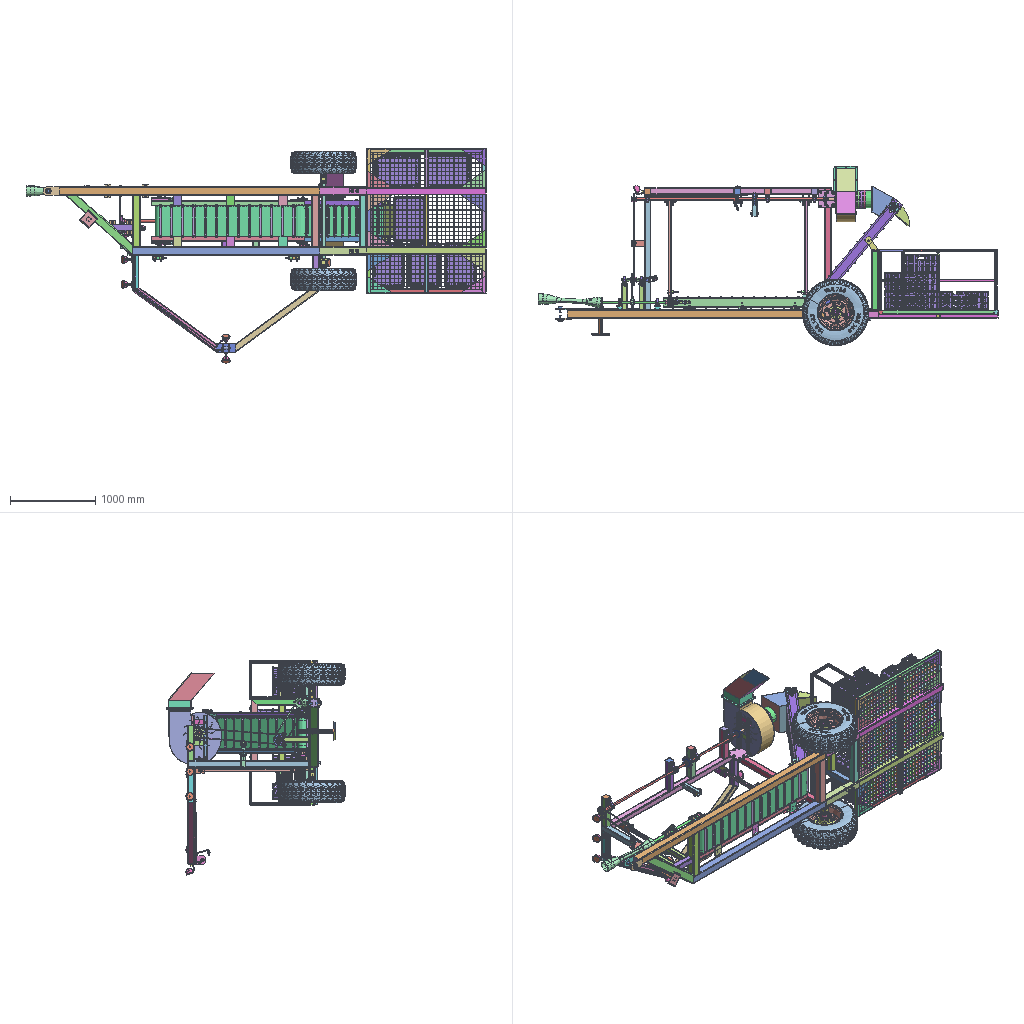Assembly | STEP file | 149 different items | 1323 placed | box 5395 x 2101 x 2512 mm
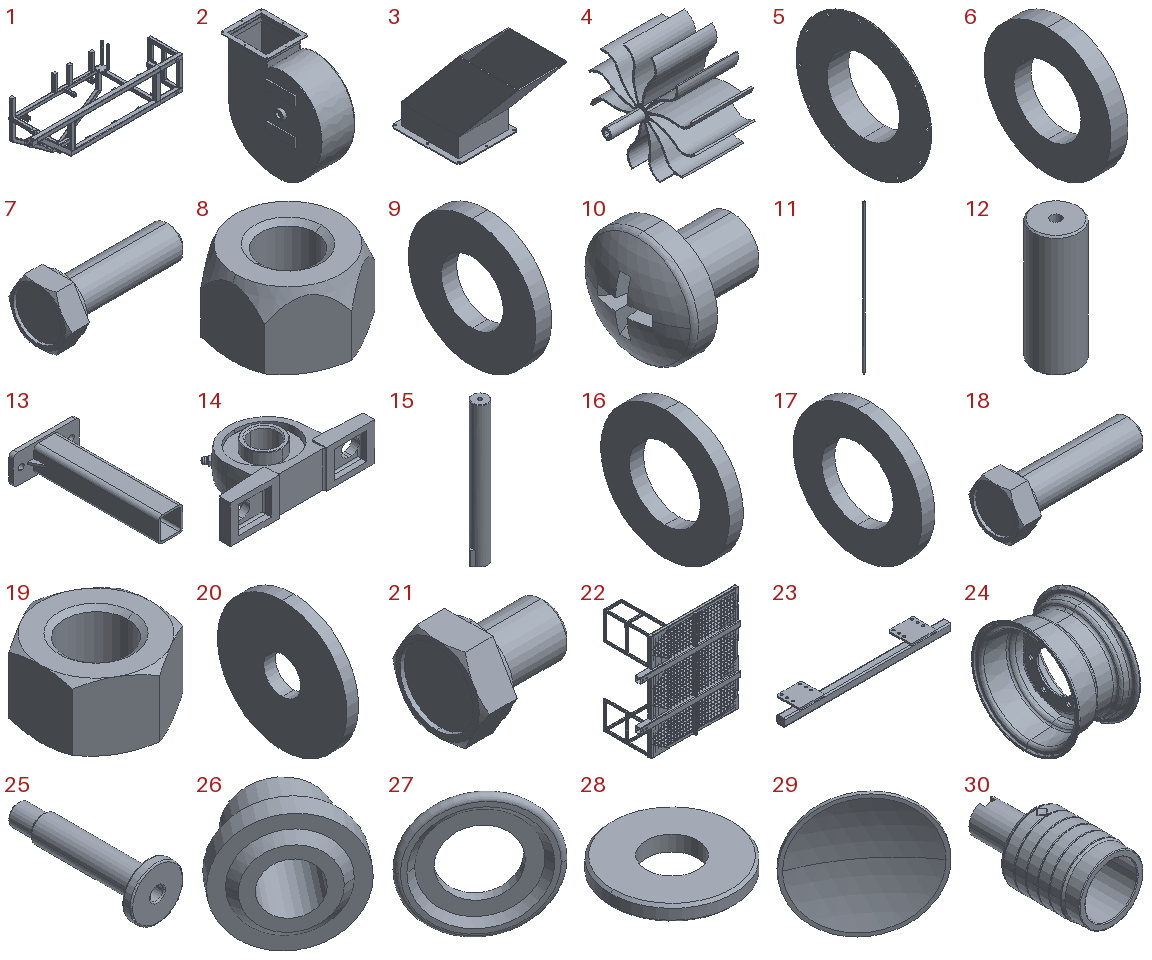Parts list (item | name | quantity | parent item | size | volume):
1 | 01_GLOWNA_RAMAV11_Default<Obrobiona> | x1 | in MAIN_FRAME_ASSEMBLY1V11 | 3794 x 1545 x 1980 mm | 40557701 mm3
2 | wentylator 1V11 | x1 | in ASSEMBLY_WENTYLATOR1V11 | 280 x 648.901 x 670.864 mm | 4184150 mm3
3 | odciag11V11 | x1 | in ASSEMBLY_WENTYLATOR1V11 | 280 x 560.788 x 414.862 mm | 1890664 mm3
4 | lopatki1V11 | x1 | in ASSEMBLY_WENTYLATOR1V11 | 347 x 377.952 x 377.952 mm | 3263464 mm3
5 | wentylator blacha dodatkowaV11 | x1 | in ASSEMBLY_WENTYLATOR1V11 | 60 x 370 x 370 mm | 388519 mm3
6 | flat washer narrow_am_B18.22M - Plain washer, 6 mm, narrow | x16 | in ASSEMBLY_WENTYLATOR1V11 | 1.75 x 13 x 13 mm | 167.412 mm3
7 | formed hex screw_am_B18.2.3.2M - Formed hex screw, M6 x 1.0 x 20 --20WN | x8 | in ASSEMBLY_WENTYLATOR1V11 | 24.15 x 11.547 x 10 mm | 885.854 mm3
8 | prevailing torque hex nut_am_AM-M6-N | x10 | in ASSEMBLY_WENTYLATOR1V11, P01_ASSEMBLY_FRUIT_HARVESTER1 | 10 x 11.547 x 6.7 mm | 433.135 mm3
9 | flat washer narrow_am_B18.22M - Plain washer, 8 mm, narrow | x12 | in ASSEMBLY_WENTYLATOR1V11 | 2.3 x 18.8 x 18.8 mm | 488.212 mm3
10 | pan cross head_am_B18.6.7M - M8 x 1.25 x 10 Type I Cross Recessed PHMS --10N | x12 | in ASSEMBLY_WENTYLATOR1V11 | 15.946 x 16 x 16 mm | 1390 mm3
11 | Shaft dia30 2280V11 | x1 | in MAIN_FRAME_ASSEMBLY1V11 | 30 x 30 x 2310 mm | 1619744 mm3
12 | SHAFT_DIA30_80V11 | x1 | in MAIN_FRAME_ASSEMBLY1V11 | 30 x 30 x 80 mm | 54791 mm3
13 | MOUNTING_BOTTOM_PROFILEV11_Default<Machined> | x2 | in ASSEMBLY_MOCOWANIE1V11 | 160 x 310 x 70 mm | 420999 mm3
14 | ucp206_01V11 | x4 | in ASSEMBLY_MOCOWANIE1V11, ASSEMBLY_MOCOWANIE2V11 | 160 x 84 x 43.2 mm | 181107 mm3
15 | SHAFT_DIA30_BOTTOM_MOUNTINGV11 | x1 | in ASSEMBLY_MOCOWANIE1V11 | 39 x 30 x 270 mm | 190340 mm3
16 | flat washer narrow_am_B18.22M - Plain washer, 16 mm, narrow | x5 | in ASSEMBLY_MOCOWANIE1V11, zlozenie mniejszego podajnika1V11 | 3.5 x 32 x 32 mm | 1956 mm3
17 | flat washer narrow_am_B18.22M - Plain washer, 14 mm, narrow | x56 | in ASSEMBLY_MOCOWANIE1V11, Assembly Ucp206V11, MAIN_FRAME_ASSEMBLY1V11, ASSEMBLY_MOCOWANIE2V11 | 2.8 x 28 x 28 mm | 1194 mm3
18 | formed hex screw_am_B18.2.3.2M - Formed hex screw, M14 x 2.0 x 50 --34WN | x4 | in ASSEMBLY_MOCOWANIE1V11 | 59.09 x 24.249 x 21 mm | 10811 mm3
19 | hex nut style 1_am_B18.2.4.1M - Hex nut, Style 1,  M14 x 2 --D-N | x16 | in ASSEMBLY_MOCOWANIE1V11, MAIN_FRAME_ASSEMBLY1V11 | 21 x 24.249 x 12.8 mm | 3392 mm3
20 | flat washer wide_am_B18.22M - Plain washer, 10 mm, wide | x1 | in ASSEMBLY_MOCOWANIE1V11 | 3.5 x 39 x 39 mm | 3841 mm3
21 | formed hex screw_am_B18.2.3.2M - Formed hex screw, M10 x 1.5 x 14 --14WN | x11 | in ASSEMBLY_MOCOWANIE1V11, zlozenie mniejszego podajnika1V11, P01_ASSEMBLY_FRUIT_HARVESTER1 | 20.63 x 18.475 x 16 mm | 2415 mm3
22 | REAR_RECEIVING_PLATFORMV11_Default<Machined> | x1 | in MAIN_FRAME_ASSEMBLY1V11 | 1600 x 805 x 1690 mm | 26046895 mm3
23 | REAR_AXIS_PROFILEV11_Default<Machined> | x1 | in REAR_AXIS_ASSEMBLY1V11 | 1070 x 150 x 60 mm | 1274604 mm3
24 | FELGA_9.00x15.3V11 | x2 | in GEAR_ASSEMBLYV11 | 254.399 x 439.355 x 439.355 mm | 2312376 mm3
25 | VALVE_1PARTV11 | x2 | in GEAR_ASSEMBLYV11 | 20 x 53 x 20 mm | 3450 mm3
26 | VALVE_2PARTV11 | x2 | in GEAR_ASSEMBLYV11 | 22.76 x 21.764 x 22 mm | 2471 mm3
27 | VALVE_3PARTV11 | x2 | in GEAR_ASSEMBLYV11 | 16.078 x 12.89 x 20 mm | 326.438 mm3
28 | VALVE_4PARTV11 | x2 | in GEAR_ASSEMBLYV11 | 24 x 24 x 3 mm | 1103 mm3
29 | VALVE_5PARTV11 | x2 | in GEAR_ASSEMBLYV11 | 5.639 x 4.467 x 7 mm | 24.483 mm3
30 | VALVE_6PARTV11 | x2 | in GEAR_ASSEMBLYV11 | 9 x 17 x 9 mm | 343.749 mm3
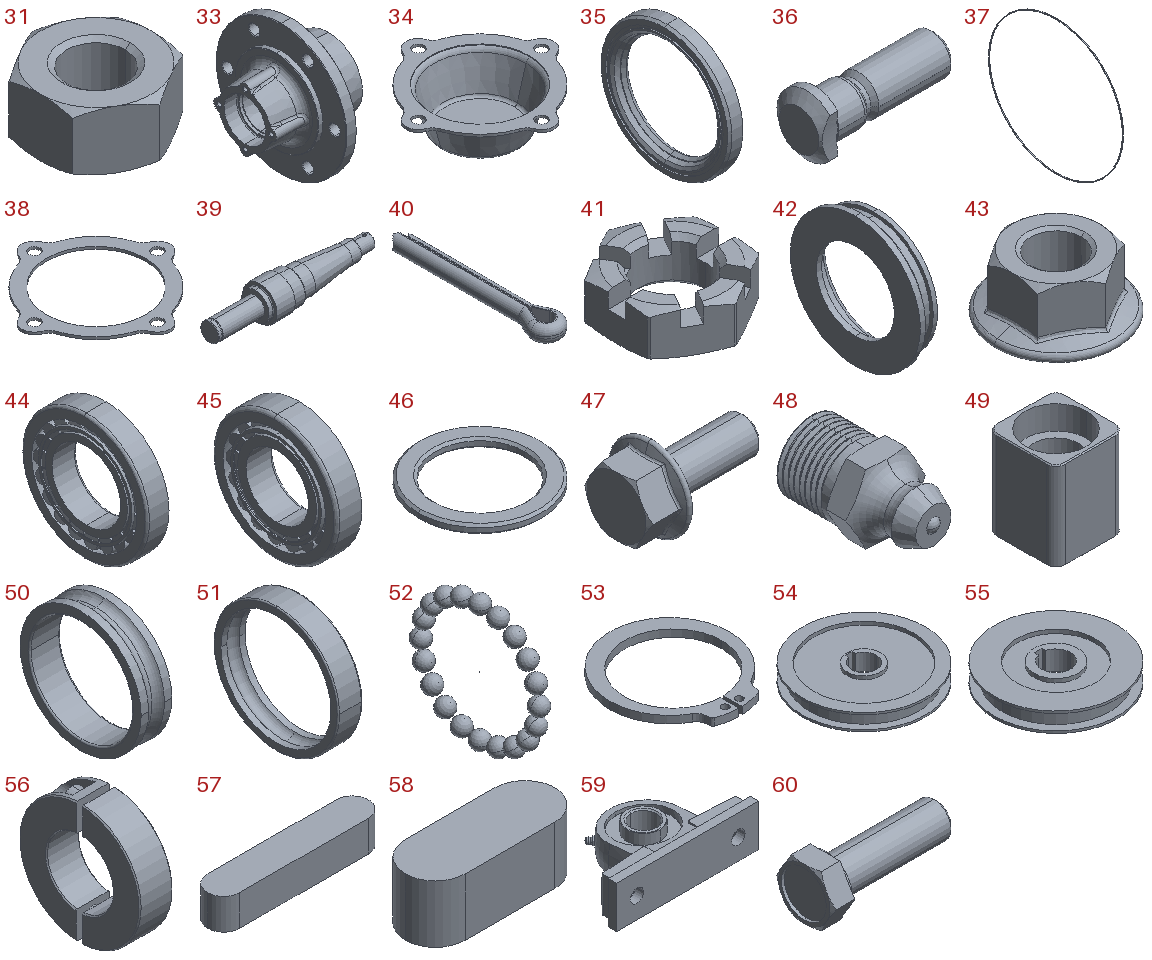31 | hex nut style 1_am_B18.2.4.1M - Hex nut, Style 1,  M10 x 1.5, with 16mm WAF --D-N | x2 | in GEAR_ASSEMBLYV11 | 16 x 18.475 x 8.4 mm | 1365 mm3
32 | OPONA_10.0-75_15.3V11 | x2 | in GEAR_ASSEMBLYV11 | - | -
33 | AXIS_HOUSING1V11 | x2 | in GEAR_ASSEMBLYV11 | 160 x 250 x 250 mm | 1786863 mm3
34 | AXIS_COVER1V11 | x2 | in GEAR_ASSEMBLYV11 | 120 x 120 x 31.5 mm | 20879 mm3
35 | SIMMERING_KORPUS1V11 | x2 | in GEAR_ASSEMBLYV11 | 10 x 95 x 95 mm | 14984 mm3
36 | SCREW_1SHAFTV11 | x12 | in GEAR_ASSEMBLYV11 | 68 x 26.359 x 30 mm | 23158 mm3
37 | USZCZELKA_SIMMERING1V11 | x2 | in GEAR_ASSEMBLYV11 | 0.5 x 78.541 x 78.541 mm | 35.939 mm3
38 | USZCZELKA1V11 | x2 | in GEAR_ASSEMBLYV11 | 120 x 120 x 2 mm | 6543 mm3
39 | SHAFT_AXIS_HOUSING1V11 | x2 | in GEAR_ASSEMBLYV11 | 349 x 75 x 75 mm | 734000 mm3
40 | SLIDER_SHAFT1V11 | x2 | in GEAR_ASSEMBLYV11 | 11.05 x 60.6 x 5.8 mm | 1645 mm3
41 | SHAFT_CAP1V11 | x2 | in GEAR_ASSEMBLYV11 | 46 x 52.616 x 18 mm | 18537 mm3
42 | AXIS_HOUSING_CLOSURE1V11 | x2 | in GEAR_ASSEMBLYV11 | 21 x 120 x 120 mm | 65717 mm3
43 | hex flange nut_am_B18.2.2.4M - Hex flange nut, M20 x 2.5 --N | x12 | in GEAR_ASSEMBLYV11 | 42.8 x 42.8 x 20 mm | 12973 mm3
44 | 30212V11 | x2 | in GEAR_ASSEMBLYV11 | 23.75 x 110 x 110 mm | 111845 mm3
45 | 30208V11 | x2 | in GEAR_ASSEMBLYV11 | 19.75 x 80 x 80 mm | 51729 mm3
46 | WASHER_DIA40_1V11 | x2 | in GEAR_ASSEMBLYV11 | 55 x 55 x 4 mm | 4178 mm3
47 | heavy hex flange screw_am_B18.2.3.9M - Heavy hex flange screw, M8 x 1.25 x 20 --20N | x8 | in GEAR_ASSEMBLYV11 | 28.1 x 18 x 18 mm | 2330 mm3
48 | KALAMITKA_1V11 | x2 | in GEAR_ASSEMBLYV11 | 11.547 x 18.49 x 10 mm | 633.492 mm3
49 | MILLED_BLOCK_FOR_AXISV11 | x2 | in REAR_AXIS_ASSEMBLY1V11 | 70 x 70 x 90 mm | 221300 mm3
50 | bearing_6908_01V11 | x8 | in bearing_6908V11 | 12 x 47.33 x 47.33 mm | 4895 mm3
51 | bearing_6908_02V11 | x8 | in bearing_6908V11 | 12 x 62 x 62 mm | 6668 mm3
52 | bearing_6908_03V11 | x8 | in bearing_6908V11 | 7.2 x 58.195 x 58.195 mm | 3909 mm3
53 | heavy duty external retaining ring_am_B27.8M - 3DM1-40 | x2 | in REAR_AXIS_ASSEMBLY1V11 | 46.312 x 50.391 x 2.8 mm | 1790 mm3
54 | Pulley 150 belt ha13v1V11 | x3 | in MAIN_FRAME_ASSEMBLY1V11 | 147 x 147 x 20 mm | 190388 mm3
55 | Pulley 150 belt ha13 v1V11 | x3 | in MAIN_FRAME_ASSEMBLY1V11, P01_ASSEMBLY_FRUIT_HARVESTER1 | 127 x 127 x 20 mm | 165003 mm3
56 | Split Shaft Collar_ Steel GN 707.2-55-B30-STV11 | x9 | in MAIN_FRAME_ASSEMBLY1V11, P01_ASSEMBLY_FRUIT_HARVESTER1 | 15 x 55 x 54.918 mm | 22142 mm3
57 | Keyway 8x40V11_Default<Machined> | x1 | in MAIN_FRAME_ASSEMBLY1V11 | 40 x 8 x 7.7 mm | 2358 mm3
58 | Keyway 8x20V11_Default<Machined> | x3 | in MAIN_FRAME_ASSEMBLY1V11 | 20 x 8 x 7.7 mm | 1126 mm3
59 | ucp206 z blacha1V11 | x4 | in Assembly Ucp206V11 | 170 x 94 x 50 mm | 262085 mm3
60 | formed hex screw_am_B18.2.3.2M - Formed hex screw, M14 x 2.0 x 45 --45WN | x20 | in Assembly Ucp206V11, MAIN_FRAME_ASSEMBLY1V11 | 54.09 x 24.249 x 21 mm | 10041 mm3
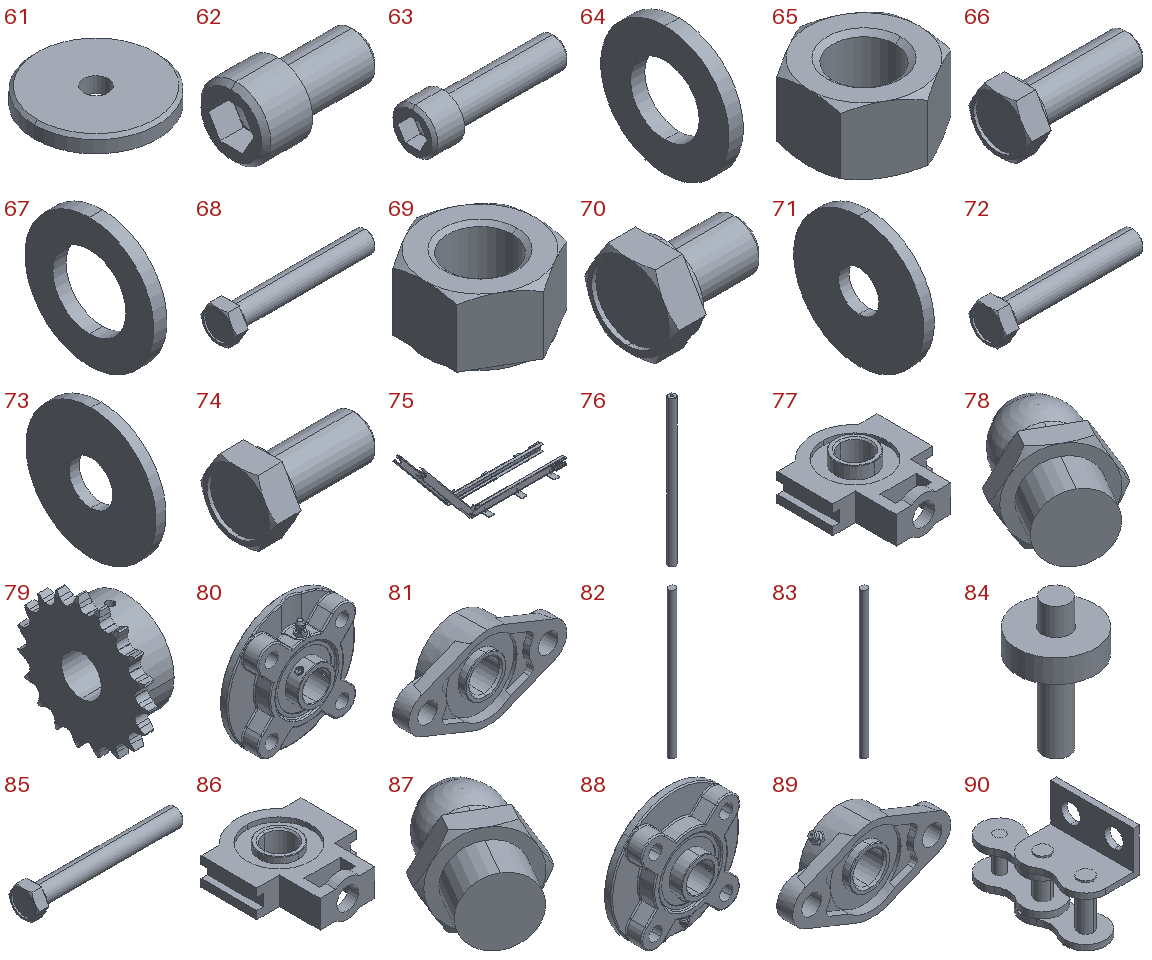61 | WASHER_DIA40V11 | x2 | in MAIN_FRAME_ASSEMBLY1V11 | 40 x 40 x 5 mm | 5970 mm3
62 | socket head cap screw_am_B18.3.1M - 12 x 1.75 x 20 Hex SHCS -- 20NHX | x3 | in MAIN_FRAME_ASSEMBLY1V11 | 32 x 18 x 18 mm | 4653 mm3
63 | socket head cap screw_am_B18.3.1M - 12 x 1.75 x 45 Hex SHCS -- 45NHX | x2 | in MAIN_FRAME_ASSEMBLY1V11 | 57 x 18 x 18 mm | 7481 mm3
64 | flat washer narrow_am_B18.22M - Plain washer, 12 mm, narrow | x16 | in MAIN_FRAME_ASSEMBLY1V11, zlozenie mniejszego podajnika1V11, P01_ASSEMBLY_FRUIT_HARVESTER1 | 2.8 x 25.4 x 25.4 mm | 1014 mm3
65 | hex nut style 1_am_B18.2.4.1M - Hex nut, Style 1,  M12 x 1.75 --D-N | x4 | in MAIN_FRAME_ASSEMBLY1V11, zlozenie mniejszego podajnika1V11 | 18 x 20.785 x 10.8 mm | 2115 mm3
66 | formed hex screw_am_B18.2.3.2M - Formed hex screw, M12 x 1.75 x 35 --35WN | x4 | in MAIN_FRAME_ASSEMBLY1V11 | 42.76 x 20.785 x 18 mm | 5908 mm3
67 | flat washer narrow_am_B18.22M - Plain washer, 20 mm, narrow | x14 | in MAIN_FRAME_ASSEMBLY1V11, P01_ASSEMBLY_FRUIT_HARVESTER1 | 4 x 39 x 39 mm | 3240 mm3
68 | formed hex screw_am_B18.2.3.2M - Formed hex screw, M20 x 2.5 x 130 --52WN | x4 | in MAIN_FRAME_ASSEMBLY1V11 | 142.88 x 34.641 x 30 mm | 49864 mm3
69 | hex nut style 1_am_B18.2.4.1M - Hex nut, Style 1,  M20 x 2.5 --W-N | x14 | in MAIN_FRAME_ASSEMBLY1V11, zlozenie mniejszego podajnika1V11 | 30 x 34.641 x 18 mm | 9548 mm3
70 | formed hex screw_am_B18.2.3.2M - Formed hex screw, M8 x 1.25 x 12 --12WN | x4 | in MAIN_FRAME_ASSEMBLY1V11, zlozenie mniejszego podajnika1V11, ASSEMBLY_MOCOWANIE2V11 | 17.5 x 15.011 x 13 mm | 1322 mm3
71 | flat washer wide_am_B18.22M - Plain washer, 14 mm, wide | x4 | in MAIN_FRAME_ASSEMBLY1V11 | 4 x 50 x 50 mm | 7097 mm3
72 | formed hex screw_am_B18.2.3.2M - Formed hex screw, M20 x 2.5 x 120 --46WN | x2 | in MAIN_FRAME_ASSEMBLY1V11 | 132.88 x 34.641 x 30 mm | 46723 mm3
73 | flat washer wide_am_B18.22M - Plain washer, 20 mm, wide | x2 | in MAIN_FRAME_ASSEMBLY1V11 | 5.1 x 66 x 66 mm | 15486 mm3
74 | formed hex screw_am_B18.2.3.2M - Formed hex screw, M24 x 3.0 x 50 --50WN | x2 | in MAIN_FRAME_ASSEMBLY1V11 | 65.44 x 41.569 x 36 mm | 38213 mm3
75 | mniejszy podajnik1V11_Default<Obrobiona> | x1 | in zlozenie mniejszego podajnika1V11 | 2807 x 780 x 1287 mm | 9743020 mm3
76 | Shaft dia 25 for feeder1V11 | x1 | in zlozenie mniejszego podajnika1V11 | 30 x 30 x 609.6 mm | 424964 mm3
77 | uct206_011V11 | x1 | in uct2061V11 | 102 x 113 x 40.7 mm | 185287 mm3
78 | uct206_021V11 | x1 | in uct2061V11 | 10.527 x 12.832 x 8 mm | 390.376 mm3
79 | 2108-191V11 | x6 | in zlozenie mniejszego podajnika1V11 | 28 x 81.525 x 81.8 mm | 74497 mm3
80 | ucfc_2051V11 | x1 | in zlozenie mniejszego podajnika1V11 | 115 x 35.698 x 115 mm | 136094 mm3
81 | ucfl2051V11 | x1 | in zlozenie mniejszego podajnika1V11 | 130 x 35.8 x 68 mm | 88119 mm3
82 | Shaft dia 25 for small 21V11 | x1 | in zlozenie mniejszego podajnika1V11 | 25 x 25 x 539.4 mm | 264777 mm3
83 | Shaft dia 25 for small 31V11 | x1 | in zlozenie mniejszego podajnika1V11 | 25 x 25 x 551.6 mm | 270766 mm3
84 | czesc do docisku llancucha1V11 | x2 | in zlozenie mniejszego podajnika1V11 | 47 x 47 x 80 mm | 37196 mm3
85 | formed hex screw_am_B18.2.3.2M - Formed hex screw, M20 x 2.5 x 160 --52WN | x2 | in zlozenie mniejszego podajnika1V11 | 172.88 x 34.641 x 30 mm | 59289 mm3
86 | Lustrouct206_011V11 | x1 | in Lustrouct2061V11 | 102 x 113 x 40.7 mm | 185287 mm3
87 | Lustrouct206_021V11 | x1 | in Lustrouct2061V11 | 10.527 x 12.832 x 8 mm | 390.376 mm3
88 | Lustroucfc_2051V11 | x1 | in zlozenie mniejszego podajnika1V11 | 115 x 35.698 x 115 mm | 136099 mm3
89 | Lustroucfl2051V11 | x1 | in zlozenie mniejszego podajnika1V11 | 130 x 35.8 x 68 mm | 88119 mm3
90 | 08b-1_e-1k2v1V11 | x127 | in Output_feeder_chain_assemblyV11 | 15.9 x 36.944 x 26.5 mm | 2584 mm3
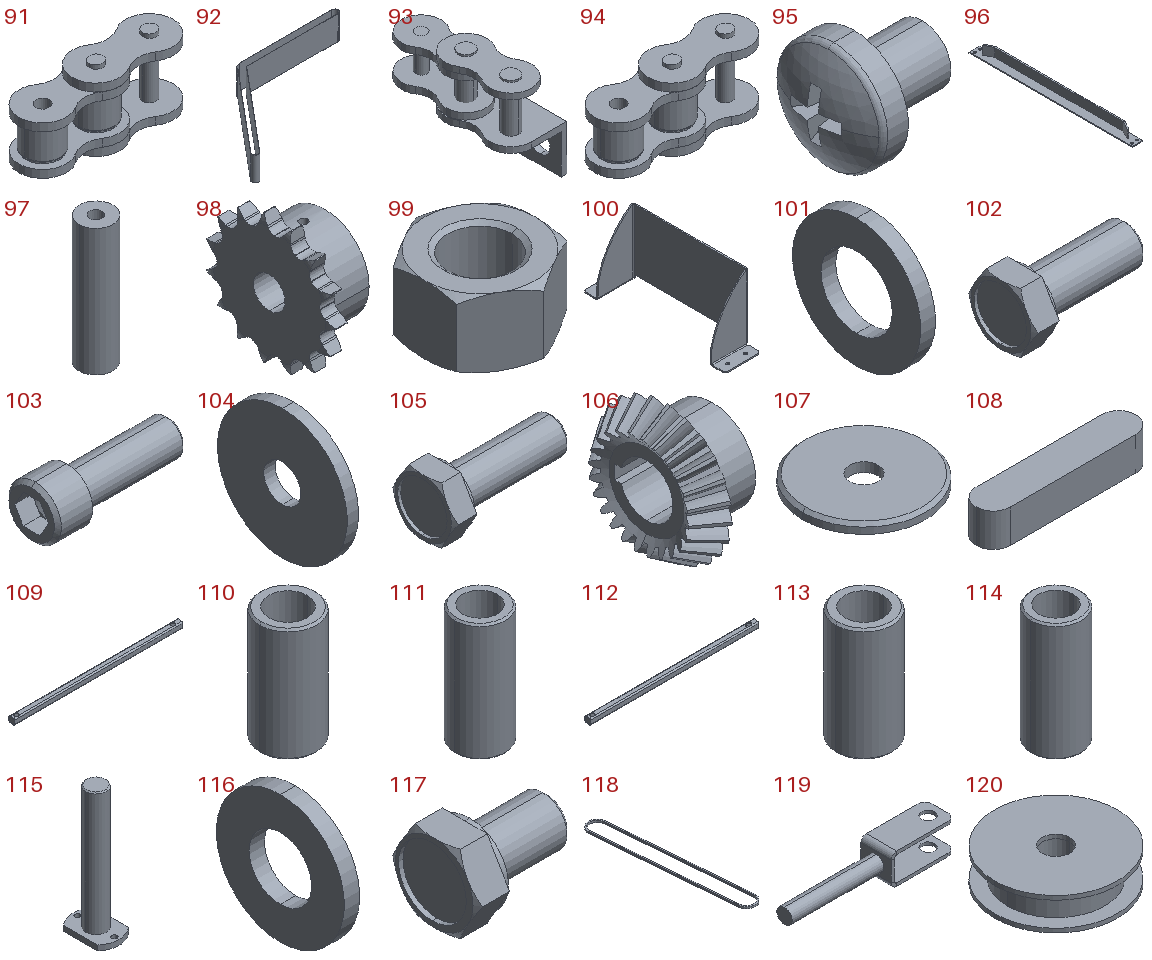91 | 08b1v1V11 | x127 | in Output_feeder_chain_assemblyV11 | 36.689 x 11.289 x 16.9 mm | 2497 mm3
92 | Copy of PART1V11 | x1 | in assembly sam podajnik 1V11 | 2633 x 1388 x 378 mm | 7453727 mm3
93 | Lustro08b-1_e-1k2v1V11 | x127 | in Mirror_Assembly_output_feeder_chainV11 | 15.9 x 36.944 x 26.5 mm | 2584 mm3
94 | Lustro08b1v1V11 | x127 | in Mirror_Assembly_output_feeder_chainV11 | 36.689 x 11.289 x 16.9 mm | 2497 mm3
95 | pan cross head_am_B18.6.7M - M5 x 0.8 x 6 Type I Cross Recessed PHMS --6N | x196 | in assembly sam podajnik 1V11 | 9.669 x 9.5 x 9.5 mm | 316.024 mm3
96 | blaszka 1 gietaV11 | x49 | in assembly sam podajnik 1V11 | 24.5 x 378 x 22 mm | 38515 mm3
97 | Shaft for belt1V11 | x3 | in zlozenie mniejszego podajnika1V11 | 80 x 80 x 300 mm | 1295907 mm3
98 | 2108-151V11 | x2 | in zlozenie mniejszego podajnika1V11 | 28 x 65.312 x 65.671 mm | 45287 mm3
99 | hex nut style 1_am_B18.2.4.1M - Hex nut, Style 1,  M16 x 2 --D-N | x4 | in zlozenie mniejszego podajnika1V11 | 24 x 27.713 x 14.8 mm | 5041 mm3
100 | ZSYP1V11 | x1 | in zlozenie mniejszego podajnika1V11 | 124 x 480 x 223 mm | 511091 mm3
101 | flat washer narrow_am_B18.22M - Plain washer, 10 mm, narrow | x27 | in zlozenie mniejszego podajnika1V11, P01_ASSEMBLY_FRUIT_HARVESTER1 | 2.3 x 20 x 20 mm | 499.195 mm3
102 | formed hex screw_am_B18.2.3.2M - Formed hex screw, M12 x 1.75 x 30 --30WN | x8 | in zlozenie mniejszego podajnika1V11 | 37.76 x 20.785 x 18 mm | 5343 mm3
103 | socket head cap screw_am_B18.3.1M - 12 x 1.75 x 35 Hex SHCS -- 35NHX | x4 | in zlozenie mniejszego podajnika1V11 | 47 x 18 x 18 mm | 6350 mm3
104 | flat washer wide_am_B18.22M - Plain washer, 8 mm, wide | x2 | in zlozenie mniejszego podajnika1V11 | 2.8 x 32 x 32 mm | 2069 mm3
105 | formed hex screw_am_B18.2.3.2M - Formed hex screw, M10 x 1.5 x 30 --30WN | x2 | in zlozenie mniejszego podajnika1V11 | 36.63 x 18.475 x 16 mm | 3671 mm3
106 | BEVEL_GEAR_24V11 | x2 | in zlozenie mniejszego podajnika1V11, ASSEMBLY_MOCOWANIE2V11 | 41.964 x 76.945 x 76.945 mm | 70048 mm3
107 | PODKLADKA_Fi39V11 | x2 | in zlozenie mniejszego podajnika1V11, ASSEMBLY_MOCOWANIE2V11 | 39 x 39 x 3 mm | 3333 mm3
108 | Keyway 8x38V11_Default<Machined> | x2 | in zlozenie mniejszego podajnika1V11, ASSEMBLY_MOCOWANIE2V11 | 37 x 8 x 7.7 mm | 2173 mm3
109 | FAN_FRAME_PROFILEV11_Default<Machined> | x1 | in Assembly_rama_wachliwaV11 | 1150 x 40 x 40 mm | 613608 mm3
110 | Bushing_dia30_len60V11 | x1 | in Assembly_rama_wachliwaV11 | 30 x 30 x 60 mm | 22516 mm3
111 | Bushing_dia30_len75V11 | x1 | in Assembly_rama_wachliwaV11 | 30 x 30 x 70 mm | 26283 mm3
112 | Mirror_FAN_FRAME_PROFILEV11_Default<Machined> | x1 | in Assembly_rama_wachliwaV11 | 1150 x 40 x 40 mm | 613608 mm3
113 | Mirror_Bushing_dia30_len60V11 | x1 | in Assembly_rama_wachliwaV11 | 30 x 30 x 60 mm | 22516 mm3
114 | Mirror_Bushing_dia30_len75V11 | x1 | in Assembly_rama_wachliwaV11 | 30 x 30 x 70 mm | 26283 mm3
115 | Locking_pinV11 | x2 | in Assembly_rama_wachliwaV11 | 30 x 45 x 125 mm | 43682 mm3
116 | flat washer narrow_am_B18.22M - Plain washer, 4 mm, narrow | x4 | in Assembly_rama_wachliwaV11 | 1.2 x 10 x 10 mm | 71.803 mm3
117 | formed hex screw_am_B18.2.3.2M - Formed hex screw, M5 x 0.8 x 8 --8WN | x4 | in Assembly_rama_wachliwaV11 | 11.65 x 9.238 x 8 mm | 337.223 mm3
118 | Pasek_klinowy2V11 | x1 | in P01_ASSEMBLY_FRUIT_HARVESTER1 | 197.097 x 1064 x 13 mm | 262478 mm3
119 | TENSION_WHEEL1V11 | x1 | in ASSEMBLY_NACIAG1V11 | 204 x 40 x 40 mm | 66853 mm3
120 | WHEEL_111V11 | x1 | in ASSEMBLY_NACIAG1V11 | 76 x 76 x 20 mm | 60554 mm3
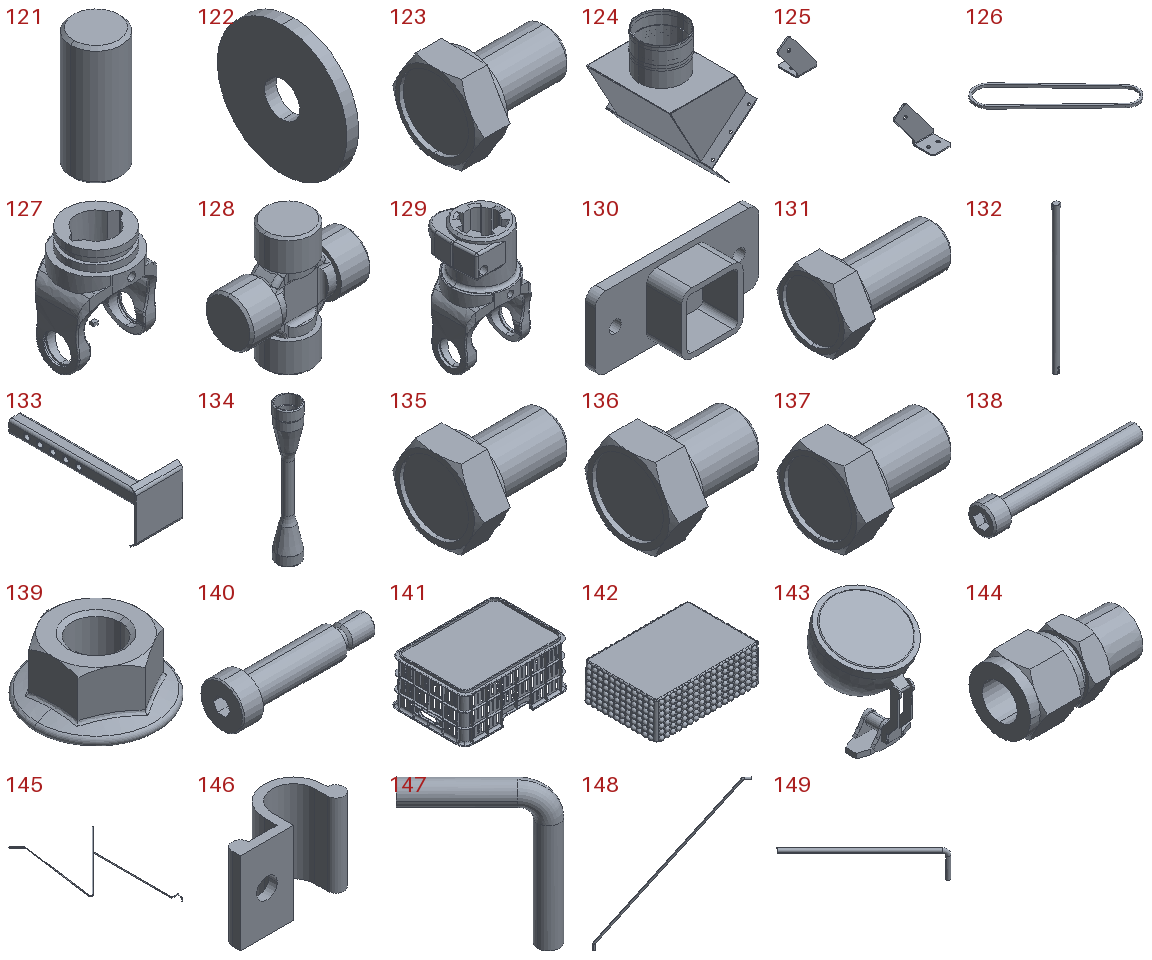121 | ROLLER_DIA171V11 | x1 | in ASSEMBLY_NACIAG1V11 | 17 x 17 x 40 mm | 9028 mm3
122 | flat washer wide_am_B18.22M - Plain washer, 6 mm, wide | x2 | in ASSEMBLY_NACIAG1V11 | 2.3 x 25.4 x 25.4 mm | 1080 mm3
123 | formed hex screw_am_B18.2.3.2M - Formed hex screw, M6 x 1.0 x 10 --10WN | x2 | in ASSEMBLY_NACIAG1V11 | 14.15 x 11.547 x 10 mm | 603.109 mm3
124 | EXHAUST1V11 | x1 | in P01_ASSEMBLY_FRUIT_HARVESTER1 | 350.686 x 484 x 530.45 mm | 1247734 mm3
125 | FEEDER_ANGLESV11 | x1 | in P01_ASSEMBLY_FRUIT_HARVESTER1 | 161.429 x 650 x 167.947 mm | 179005 mm3
126 | Pasek_klinowy3V11 | x1 | in P01_ASSEMBLY_FRUIT_HARVESTER1 | 497.285 x 498.317 x 13 mm | 184721 mm3
127 | CARDAN_1PARTV11 | x2 | in P01_ASSEMBLY_FRUIT_HARVESTER1 | 61.98 x 55.8 x 84.032 mm | 60025 mm3
128 | CARDAN_COUPLING1V11 | x2 | in P01_ASSEMBLY_FRUIT_HARVESTER1 | 55 x 22 x 55 mm | 30051 mm3
129 | CARDAN_3PARTV11 | x2 | in P01_ASSEMBLY_FRUIT_HARVESTER1 | 61.98 x 59.195 x 111.032 mm | 98715 mm3
130 | BEARING_PROFILE1V11_Default<Machined> | x2 | in ASSEMBLY_MOCOWANIE2V11 | 160 x 44.5 x 70 mm | 144609 mm3
131 | formed hex screw_am_B18.2.3.2M - Formed hex screw, M14 x 2.0 x 30 --30WN | x4 | in ASSEMBLY_MOCOWANIE2V11 | 39.09 x 24.249 x 21 mm | 7732 mm3
132 | SHAFT_DIA30_CARDANV11 | x1 | in ASSEMBLY_MOCOWANIE2V11 | 36.032 x 30 x 800 mm | 565605 mm3
133 | STOPA_KOMBAJNV11_Default<Obrobiona> | x1 | in P01_ASSEMBLY_FRUIT_HARVESTER1 | 145 x 445 x 162.836 mm | 371742 mm3
134 | SHAFT_DIA30_CARDAN2V11 | x1 | in P01_ASSEMBLY_FRUIT_HARVESTER1 | 126.77 x 126.77 x 738.528 mm | 1857517 mm3
135 | formed hex screw_am_B18.2.3.2M - Formed hex screw, M10 x 1.5 x 16 --16WN | x9 | in P01_ASSEMBLY_FRUIT_HARVESTER1 | 22.63 x 18.475 x 16 mm | 2572 mm3
136 | formed hex screw_am_B18.2.3.2M - Formed hex screw, M12 x 1.75 x 16 --16WN | x4 | in P01_ASSEMBLY_FRUIT_HARVESTER1 | 23.76 x 20.785 x 18 mm | 3759 mm3
137 | formed hex screw_am_B18.2.3.2M - Formed hex screw, M20 x 2.5 x 30 --30WN | x6 | in P01_ASSEMBLY_FRUIT_HARVESTER1 | 42.88 x 34.641 x 30 mm | 18448 mm3
138 | socket head cap screw_am_B18.3.1M - 6 x 1.0 x 50 Hex SHCS -- 24NHX | x2 | in P01_ASSEMBLY_FRUIT_HARVESTER1 | 56 x 10 x 10 mm | 1800 mm3
139 | hex flange nut_am_B18.2.2.4M - Hex flange nut, M12 x 1.75 --N | x1 | in P01_ASSEMBLY_FRUIT_HARVESTER1 | 26 x 26 x 12 mm | 2889 mm3
140 | socket head shoulder screw2_am_B18.3.3M - 16 x 50 SHSS --N | x1 | in P01_ASSEMBLY_FRUIT_HARVESTER1 | 79.4 x 24 x 24 mm | 16413 mm3
141 | SKRZYNIA_OWOCE1V11 | x10 | in P01_ASSEMBLY_FRUIT_HARVESTER1, ASSEMBLY_SKRZYNIA_OWOCE1V11 | 530 x 380 x 224 mm | 1306449 mm3
142 | CHERRIES_TO_CRATE1V11 | x6 | in ASSEMBLY_SKRZYNIA_OWOCE1V11 | 479.554 x 339.624 x 170 mm | 24539248 mm3
143 | ZAROWKA_MALA_01V11 | x7 | in P01_ASSEMBLY_FRUIT_HARVESTER1 | 96.622 x 102.595 x 127.367 mm | 131229 mm3
144 | straight fittingV11_.50 TUBE X .38 NPT | x1 | in Tube_4-P01_ASSEMBLY_KOMBAJN_OWOCOWYV11 | 43.434 x 25.663 x 22.225 mm | 9265 mm3
145 | Tube-500X083^Tube_4-P01_ASSEMBLY_KOMBAJN_OWOCOWYV11_Tube .500in OD X .083in Wall | x1 | in Tube_4-P01_ASSEMBLY_KOMBAJN_OWOCOWYV11 | 2410 x 962.272 x 1741 mm | 310969 mm3
146 | tubing_clipV11_6.01 - 12.70mm Dia | x4 | in P01_ASSEMBLY_FRUIT_HARVESTER1 | 34.48 x 15.54 x 25.4 mm | 3707 mm3
147 | Tube-500X095_1^Tube_6-P01_ASSEMBLY_KOMBAJN_OWOCOWY-003V11_Tube .500in OD X .095in Wall | x1 | in Tube_6-P01_ASSEMBLY_KOMBAJN_OWOCOWY-003V11 | 55.673 x 55.673 x 82.885 mm | 10488 mm3
148 | Tube-500X095_2^Tube_6-P01_ASSEMBLY_KOMBAJN_OWOCOWY-003V11_Tube .500in OD X .095in Wall | x1 | in Tube_6-P01_ASSEMBLY_KOMBAJN_OWOCOWY-003V11 | 548.949 x 534.807 x 1006 mm | 99272 mm3
149 | Tube-500X095_3^Tube_6-P01_ASSEMBLY_KOMBAJN_OWOCOWY-003V11_Tube .500in OD X .095in Wall | x1 | in Tube_6-P01_ASSEMBLY_KOMBAJN_OWOCOWY-003V11 | 297.218 x 297.218 x 88.076 mm | 37531 mm3
Placements (level | parent | child | x y z in mm | rotation matrix by rows), first 115 of 1358 lines:
1 | P01_ASSEMBLY_FRUIT_HARVESTER1 | MAIN_FRAME_ASSEMBLY1V11 | -0.0 -0.0 -0.0 | 1 0 0 0 1 0 0 0 1
2 | MAIN_FRAME_ASSEMBLY1V11 | 01_GLOWNA_RAMAV11_Default<Obrobiona> | -0.0 -0.0 -0.0 | 1 0 0 0 1 0 0 0 1
2 | MAIN_FRAME_ASSEMBLY1V11 | ASSEMBLY_WENTYLATOR1V11 | 1379.726 1521.485 -597.7 | 0 0 1 0 1 0 -1 0 0
3 | ASSEMBLY_WENTYLATOR1V11 | wentylator 1V11 | -534.7 53.615 703.764 | 0 0 -1 0 1 0 1 0 0
3 | ASSEMBLY_WENTYLATOR1V11 | odciag11V11 | -534.7 53.615 703.764 | 0 0 -1 0 1 0 1 0 0
3 | ASSEMBLY_WENTYLATOR1V11 | lopatki1V11 | -555.577 -373.293 703.764 | 0 -0.9474 -0.3201 0 0.3201 -0.9474 1 0 0
3 | ASSEMBLY_WENTYLATOR1V11 | wentylator blacha dodatkowaV11 | -534.7 53.615 703.764 | 0 0 -1 0 1 0 1 0 0
3 | ASSEMBLY_WENTYLATOR1V11 | flat washer narrow_am_B18.22M - Plain washer, 6 mm, narrow | -541.7 199.705 577.521 | 1 0 0 0 1 0 0 0 1
3 | ASSEMBLY_WENTYLATOR1V11 | flat washer narrow_am_B18.22M - Plain washer, 6 mm, narrow | -534.7 199.705 577.521 | -1 0 0 0 -0.3818 0.9242 0 0.9242 0.3818
3 | ASSEMBLY_WENTYLATOR1V11 | formed hex screw_am_B18.2.3.2M - Formed hex screw, M6 x 1.0 x 20 --20WN | -547.6 199.705 577.521 | 1 0 0 0 1 0 0 0 1
3 | ASSEMBLY_WENTYLATOR1V11 | prevailing torque hex nut_am_AM-M6-N | -526.25 199.705 577.521 | 0 0 1 0 1 0 -1 0 -0
3 | ASSEMBLY_WENTYLATOR1V11 | prevailing torque hex nut_am_AM-M6-N | -526.25 53.615 830.007 | 0 0 1 0 1 0 -1 0 -0
3 | ASSEMBLY_WENTYLATOR1V11 | prevailing torque hex nut_am_AM-M6-N | -526.25 -92.475 830.007 | 0 0 1 0 1 0 -1 0 -0
3 | ASSEMBLY_WENTYLATOR1V11 | prevailing torque hex nut_am_AM-M6-N | -526.25 -92.475 703.764 | 0 0 1 0 1 0 -1 0 -0
3 | ASSEMBLY_WENTYLATOR1V11 | prevailing torque hex nut_am_AM-M6-N | -526.25 -92.475 577.521 | 0 0 1 0 1 0 -1 0 -0
3 | ASSEMBLY_WENTYLATOR1V11 | prevailing torque hex nut_am_AM-M6-N | -526.25 53.615 577.521 | 0 0 1 0 1 0 -1 0 -0
3 | ASSEMBLY_WENTYLATOR1V11 | prevailing torque hex nut_am_AM-M6-N | -526.25 199.705 703.764 | 0 0 1 0 1 0 -1 0 -0
3 | ASSEMBLY_WENTYLATOR1V11 | prevailing torque hex nut_am_AM-M6-N | -526.25 199.705 830.007 | 0 0 1 0 1 0 -1 0 -0
3 | ASSEMBLY_WENTYLATOR1V11 | flat washer narrow_am_B18.22M - Plain washer, 6 mm, narrow | -534.7 53.615 830.007 | -1 0 0 0 -0.3818 0.9242 0 0.9242 0.3818
3 | ASSEMBLY_WENTYLATOR1V11 | flat washer narrow_am_B18.22M - Plain washer, 6 mm, narrow | -534.7 -92.475 830.007 | -1 0 0 0 -0.3818 0.9242 0 0.9242 0.3818
3 | ASSEMBLY_WENTYLATOR1V11 | flat washer narrow_am_B18.22M - Plain washer, 6 mm, narrow | -534.7 -92.475 703.764 | -1 0 0 0 -0.3818 0.9242 0 0.9242 0.3818
3 | ASSEMBLY_WENTYLATOR1V11 | flat washer narrow_am_B18.22M - Plain washer, 6 mm, narrow | -534.7 -92.475 577.521 | -1 0 0 0 -0.3818 0.9242 0 0.9242 0.3818
3 | ASSEMBLY_WENTYLATOR1V11 | flat washer narrow_am_B18.22M - Plain washer, 6 mm, narrow | -534.7 53.615 577.521 | -1 0 0 0 -0.3818 0.9242 0 0.9242 0.3818
3 | ASSEMBLY_WENTYLATOR1V11 | flat washer narrow_am_B18.22M - Plain washer, 6 mm, narrow | -534.7 199.705 703.764 | -1 0 0 0 -0.3818 0.9242 0 0.9242 0.3818
3 | ASSEMBLY_WENTYLATOR1V11 | flat washer narrow_am_B18.22M - Plain washer, 6 mm, narrow | -534.7 199.705 830.007 | -1 0 0 0 -0.3818 0.9242 0 0.9242 0.3818
3 | ASSEMBLY_WENTYLATOR1V11 | flat washer narrow_am_B18.22M - Plain washer, 6 mm, narrow | -541.7 53.615 830.007 | 1 0 0 0 1 0 0 0 1
3 | ASSEMBLY_WENTYLATOR1V11 | flat washer narrow_am_B18.22M - Plain washer, 6 mm, narrow | -541.7 -92.475 830.007 | 1 0 0 0 1 0 0 0 1
3 | ASSEMBLY_WENTYLATOR1V11 | flat washer narrow_am_B18.22M - Plain washer, 6 mm, narrow | -541.7 -92.475 703.764 | 1 0 0 0 1 0 0 0 1
3 | ASSEMBLY_WENTYLATOR1V11 | flat washer narrow_am_B18.22M - Plain washer, 6 mm, narrow | -541.7 -92.475 577.521 | 1 0 0 0 1 0 0 0 1
3 | ASSEMBLY_WENTYLATOR1V11 | flat washer narrow_am_B18.22M - Plain washer, 6 mm, narrow | -541.7 53.615 577.521 | 1 0 0 0 1 0 0 0 1
3 | ASSEMBLY_WENTYLATOR1V11 | flat washer narrow_am_B18.22M - Plain washer, 6 mm, narrow | -541.7 199.705 703.764 | 1 0 0 0 1 0 0 0 1
3 | ASSEMBLY_WENTYLATOR1V11 | flat washer narrow_am_B18.22M - Plain washer, 6 mm, narrow | -541.7 199.705 830.007 | 1 0 0 0 1 0 0 0 1
3 | ASSEMBLY_WENTYLATOR1V11 | formed hex screw_am_B18.2.3.2M - Formed hex screw, M6 x 1.0 x 20 --20WN | -547.6 53.615 830.007 | 1 0 0 0 1 0 0 0 1
3 | ASSEMBLY_WENTYLATOR1V11 | formed hex screw_am_B18.2.3.2M - Formed hex screw, M6 x 1.0 x 20 --20WN | -547.6 -92.475 830.007 | 1 0 0 0 1 0 0 0 1
3 | ASSEMBLY_WENTYLATOR1V11 | formed hex screw_am_B18.2.3.2M - Formed hex screw, M6 x 1.0 x 20 --20WN | -547.6 -92.475 703.764 | 1 0 0 0 1 0 0 0 1
3 | ASSEMBLY_WENTYLATOR1V11 | formed hex screw_am_B18.2.3.2M - Formed hex screw, M6 x 1.0 x 20 --20WN | -547.6 -92.475 577.521 | 1 0 0 0 1 0 0 0 1
3 | ASSEMBLY_WENTYLATOR1V11 | formed hex screw_am_B18.2.3.2M - Formed hex screw, M6 x 1.0 x 20 --20WN | -547.6 53.615 577.521 | 1 0 0 0 1 0 0 0 1
3 | ASSEMBLY_WENTYLATOR1V11 | formed hex screw_am_B18.2.3.2M - Formed hex screw, M6 x 1.0 x 20 --20WN | -547.6 199.705 703.764 | 1 0 0 0 1 0 0 0 1
3 | ASSEMBLY_WENTYLATOR1V11 | formed hex screw_am_B18.2.3.2M - Formed hex screw, M6 x 1.0 x 20 --20WN | -547.6 199.705 830.007 | 1 0 0 0 1 0 0 0 1
3 | ASSEMBLY_WENTYLATOR1V11 | flat washer narrow_am_B18.22M - Plain washer, 8 mm, narrow | -151.696 -28.069 818.764 | 0 0 1 0 1 0 -1 0 -0
3 | ASSEMBLY_WENTYLATOR1V11 | pan cross head_am_B18.6.7M - M8 x 1.25 x 10 Type I Cross Recessed PHMS --10N | -151.696 -28.069 827.064 | 0 0 1 0 1 0 -1 0 -0
3 | ASSEMBLY_WENTYLATOR1V11 | flat washer narrow_am_B18.22M - Plain washer, 8 mm, narrow | -326.411 -18.086 818.764 | 0 -0.866 0.5 0 0.5 0.866 -1 0 -0
3 | ASSEMBLY_WENTYLATOR1V11 | flat washer narrow_am_B18.22M - Plain washer, 8 mm, narrow | -394.016 -78.381 818.764 | 0 -1 0 0 0 1 -1 0 -0
3 | ASSEMBLY_WENTYLATOR1V11 | flat washer narrow_am_B18.22M - Plain washer, 8 mm, narrow | -422.415 -164.401 818.764 | 0 -0.866 -0.5 0 -0.5 0.866 -1 0 0
3 | ASSEMBLY_WENTYLATOR1V11 | flat washer narrow_am_B18.22M - Plain washer, 8 mm, narrow | -403.999 -253.096 818.764 | 0 -0.5 -0.866 0 -0.866 0.5 -1 0 0
3 | ASSEMBLY_WENTYLATOR1V11 | flat washer narrow_am_B18.22M - Plain washer, 8 mm, narrow | -343.704 -320.701 818.764 | 0 0 -1 0 -1 0 -1 0 0
3 | ASSEMBLY_WENTYLATOR1V11 | flat washer narrow_am_B18.22M - Plain washer, 8 mm, narrow | -257.684 -349.1 818.764 | 0 0.5 -0.866 0 -0.866 -0.5 -1 0 0
3 | ASSEMBLY_WENTYLATOR1V11 | flat washer narrow_am_B18.22M - Plain washer, 8 mm, narrow | -168.989 -330.685 818.764 | 0 0.866 -0.5 0 -0.5 -0.866 -1 0 0
3 | ASSEMBLY_WENTYLATOR1V11 | flat washer narrow_am_B18.22M - Plain washer, 8 mm, narrow | -101.384 -270.389 818.764 | 0 1 0 0 0 -1 -1 0 0
3 | ASSEMBLY_WENTYLATOR1V11 | flat washer narrow_am_B18.22M - Plain washer, 8 mm, narrow | -72.985 -184.369 818.764 | 0 0.866 0.5 0 0.5 -0.866 -1 0 -0
3 | ASSEMBLY_WENTYLATOR1V11 | flat washer narrow_am_B18.22M - Plain washer, 8 mm, narrow | -91.4 -95.674 818.764 | 0 0.5 0.866 0 0.866 -0.5 -1 0 -0
3 | ASSEMBLY_WENTYLATOR1V11 | flat washer narrow_am_B18.22M - Plain washer, 8 mm, narrow | -237.716 0.3299 818.764 | 0 -0.5 0.866 0 0.866 0.5 -1 0 -0
3 | ASSEMBLY_WENTYLATOR1V11 | pan cross head_am_B18.6.7M - M8 x 1.25 x 10 Type I Cross Recessed PHMS --10N | -326.411 -18.086 827.064 | 0 -0.866 0.5 0 0.5 0.866 -1 0 -0
3 | ASSEMBLY_WENTYLATOR1V11 | pan cross head_am_B18.6.7M - M8 x 1.25 x 10 Type I Cross Recessed PHMS --10N | -394.016 -78.381 827.064 | 0 -1 0 0 0 1 -1 0 -0
3 | ASSEMBLY_WENTYLATOR1V11 | pan cross head_am_B18.6.7M - M8 x 1.25 x 10 Type I Cross Recessed PHMS --10N | -422.415 -164.401 827.064 | 0 -0.866 -0.5 0 -0.5 0.866 -1 0 0
3 | ASSEMBLY_WENTYLATOR1V11 | pan cross head_am_B18.6.7M - M8 x 1.25 x 10 Type I Cross Recessed PHMS --10N | -403.999 -253.096 827.064 | 0 -0.5 -0.866 0 -0.866 0.5 -1 0 0
3 | ASSEMBLY_WENTYLATOR1V11 | pan cross head_am_B18.6.7M - M8 x 1.25 x 10 Type I Cross Recessed PHMS --10N | -343.704 -320.701 827.064 | 0 0 -1 0 -1 0 -1 0 0
3 | ASSEMBLY_WENTYLATOR1V11 | pan cross head_am_B18.6.7M - M8 x 1.25 x 10 Type I Cross Recessed PHMS --10N | -257.684 -349.1 827.064 | 0 0.5 -0.866 0 -0.866 -0.5 -1 0 0
3 | ASSEMBLY_WENTYLATOR1V11 | pan cross head_am_B18.6.7M - M8 x 1.25 x 10 Type I Cross Recessed PHMS --10N | -168.989 -330.685 827.064 | 0 0.866 -0.5 0 -0.5 -0.866 -1 0 0
3 | ASSEMBLY_WENTYLATOR1V11 | pan cross head_am_B18.6.7M - M8 x 1.25 x 10 Type I Cross Recessed PHMS --10N | -101.384 -270.389 827.064 | 0 1 0 0 0 -1 -1 0 0
3 | ASSEMBLY_WENTYLATOR1V11 | pan cross head_am_B18.6.7M - M8 x 1.25 x 10 Type I Cross Recessed PHMS --10N | -72.985 -184.369 827.064 | 0 0.866 0.5 0 0.5 -0.866 -1 0 -0
3 | ASSEMBLY_WENTYLATOR1V11 | pan cross head_am_B18.6.7M - M8 x 1.25 x 10 Type I Cross Recessed PHMS --10N | -91.4 -95.674 827.064 | 0 0.5 0.866 0 0.866 -0.5 -1 0 -0
3 | ASSEMBLY_WENTYLATOR1V11 | pan cross head_am_B18.6.7M - M8 x 1.25 x 10 Type I Cross Recessed PHMS --10N | -237.716 0.3299 827.064 | 0 -0.5 0.866 0 0.866 0.5 -1 0 -0
2 | MAIN_FRAME_ASSEMBLY1V11 | Shaft dia30 2280V11 | 1852.49 1347.1 -350.0 | 0 0 -1 0.4435 -0.8963 0 -0.8963 -0.4435 0
2 | MAIN_FRAME_ASSEMBLY1V11 | SHAFT_DIA30_80V11 | 857.49 1310.0 -1840.0 | 0 0 -1 0 1 0 1 0 0
2 | MAIN_FRAME_ASSEMBLY1V11 | ASSEMBLY_MOCOWANIE1V11 | -202.51 236.438 -369.824 | 0 0 -1 0 1 0 1 0 0
3 | ASSEMBLY_MOCOWANIE1V11 | MOUNTING_BOTTOM_PROFILEV11_Default<Machined> | -57.273 -53.543 310.0 | 1 0 0 0 1 0 0 0 1
3 | ASSEMBLY_MOCOWANIE1V11 | ucp206_01V11 | -57.273 166.462 310.0 | 1 0 0 0 1 0 0 0 1
3 | ASSEMBLY_MOCOWANIE1V11 | MOUNTING_BOTTOM_PROFILEV11_Default<Machined> | -57.273 -53.543 110.0 | 1 0 0 0 1 0 0 0 1
3 | ASSEMBLY_MOCOWANIE1V11 | ucp206_01V11 | -57.273 166.462 110.0 | 1 0 0 0 1 0 0 0 1
3 | ASSEMBLY_MOCOWANIE1V11 | SHAFT_DIA30_BOTTOM_MOUNTINGV11 | -57.273 166.462 62.2 | 1 0 0 0 1 0 0 0 1
3 | ASSEMBLY_MOCOWANIE1V11 | flat washer narrow_am_B18.22M - Plain washer, 16 mm, narrow | 3.227 139.562 110.0 | 0 0.9683 -0.2499 -1 0 0 0 0.2499 0.9683
3 | ASSEMBLY_MOCOWANIE1V11 | flat washer narrow_am_B18.22M - Plain washer, 14 mm, narrow | 3.227 113.562 110.0 | 0 -1 0 1 0 0 0 0 1
3 | ASSEMBLY_MOCOWANIE1V11 | flat washer narrow_am_B18.22M - Plain washer, 14 mm, narrow | -117.773 113.562 110.0 | 0 -1 0 1 0 0 0 0 1
3 | ASSEMBLY_MOCOWANIE1V11 | flat washer narrow_am_B18.22M - Plain washer, 14 mm, narrow | -117.773 113.562 310.0 | 0 -1 0 1 0 0 0 0 1
3 | ASSEMBLY_MOCOWANIE1V11 | flat washer narrow_am_B18.22M - Plain washer, 14 mm, narrow | 3.227 113.562 310.0 | 0 -1 0 1 0 0 0 0 1
3 | ASSEMBLY_MOCOWANIE1V11 | flat washer narrow_am_B18.22M - Plain washer, 14 mm, narrow | 3.227 139.562 310.0 | 0 1 0 -1 0 0 0 0 1
3 | ASSEMBLY_MOCOWANIE1V11 | flat washer narrow_am_B18.22M - Plain washer, 14 mm, narrow | -117.773 139.562 310.0 | 0 1 0 -1 0 0 0 0 1
3 | ASSEMBLY_MOCOWANIE1V11 | flat washer narrow_am_B18.22M - Plain washer, 14 mm, narrow | -117.773 139.562 110.0 | 0 0.4522 0.8919 -1 0 0 0 -0.8919 0.4522
3 | ASSEMBLY_MOCOWANIE1V11 | formed hex screw_am_B18.2.3.2M - Formed hex screw, M14 x 2.0 x 50 --34WN | 3.227 151.452 310.0 | 0 1 0 -1 0 0 0 0 1
3 | ASSEMBLY_MOCOWANIE1V11 | formed hex screw_am_B18.2.3.2M - Formed hex screw, M14 x 2.0 x 50 --34WN | -117.773 151.452 310.0 | 0 1 0 -1 0 0 0 0 1
3 | ASSEMBLY_MOCOWANIE1V11 | formed hex screw_am_B18.2.3.2M - Formed hex screw, M14 x 2.0 x 50 --34WN | -117.773 151.452 110.0 | 0 1 0 -1 0 0 0 0 1
3 | ASSEMBLY_MOCOWANIE1V11 | formed hex screw_am_B18.2.3.2M - Formed hex screw, M14 x 2.0 x 50 --34WN | 3.227 152.152 110.0 | 0 1 0 -1 0 0 0 0 1
3 | ASSEMBLY_MOCOWANIE1V11 | hex nut style 1_am_B18.2.4.1M - Hex nut, Style 1,  M14 x 2 --D-N | 3.227 97.962 110.0 | 1 0 0 0 0 -1 0 1 0
3 | ASSEMBLY_MOCOWANIE1V11 | hex nut style 1_am_B18.2.4.1M - Hex nut, Style 1,  M14 x 2 --D-N | -117.773 97.962 110.0 | 1 0 0 0 0 -1 0 1 0
3 | ASSEMBLY_MOCOWANIE1V11 | hex nut style 1_am_B18.2.4.1M - Hex nut, Style 1,  M14 x 2 --D-N | -117.773 97.962 310.0 | 1 0 0 0 0 -1 0 1 0
3 | ASSEMBLY_MOCOWANIE1V11 | hex nut style 1_am_B18.2.4.1M - Hex nut, Style 1,  M14 x 2 --D-N | 3.227 97.962 310.0 | 1 0 0 0 0 -1 0 1 0
3 | ASSEMBLY_MOCOWANIE1V11 | flat washer wide_am_B18.22M - Plain washer, 10 mm, wide | -57.273 166.462 332.2 | 0 0 1 0 1 0 -1 0 0
3 | ASSEMBLY_MOCOWANIE1V11 | formed hex screw_am_B18.2.3.2M - Formed hex screw, M10 x 1.5 x 14 --14WN | -57.273 166.462 342.33 | 0 0 1 0 1 0 -1 0 0
2 | MAIN_FRAME_ASSEMBLY1V11 | REAR_RECEIVING_PLATFORMV11_Default<Machined> | 3067.49 -0.0 -700.0 | 1 0 0 0 1 0 0 0 1
2 | MAIN_FRAME_ASSEMBLY1V11 | REAR_AXIS_ASSEMBLY1V11 | 3217.49 116.541 -246.807 | 0 0 -1 0 1 0 1 0 0
3 | REAR_AXIS_ASSEMBLY1V11 | REAR_AXIS_PROFILEV11_Default<Machined> | -103.193 -36.541 1255.0 | 1 0 0 0 1 0 0 0 1
3 | REAR_AXIS_ASSEMBLY1V11 | GEAR_ASSEMBLYV11 | -780.724 297.214 1039.542 | -1 0 0 0 -0.3201 -0.9474 0 -0.9474 0.3201
4 | GEAR_ASSEMBLYV11 | FELGA_9.00x15.3V11 | 8.219 -78.084 442.005 | 1 0 0 0 -1 0 0 0 -1
4 | GEAR_ASSEMBLYV11 | VALVE_1PARTV11 | 73.277 -271.786 442.36 | 0.7871 0.6157 -0.03879 -0.6149 0.788 0.0303 0.04922 0 0.9988
4 | GEAR_ASSEMBLYV11 | VALVE_2PARTV11 | 65.736 -262.355 441.281 | 0.9922 0.006081 -0.1244 0.006081 0.9952 0.09717 0.1244 -0.09717 0.9875
4 | GEAR_ASSEMBLYV11 | VALVE_3PARTV11 | 72.999 -255.232 442.005 | 1 0 0 0 1 0 0 0 1
4 | GEAR_ASSEMBLYV11 | VALVE_4PARTV11 | 77.745 -254.338 442.005 | 0.7115 -0.3387 0.6157 -0.5559 0.2646 0.788 -0.4299 -0.9029 0
4 | GEAR_ASSEMBLYV11 | VALVE_5PARTV11 | 101.454 -223.992 442.005 | 0.9751 0.01942 0.2207 0.01942 0.9848 -0.1725 -0.2207 0.1725 0.96
4 | GEAR_ASSEMBLYV11 | VALVE_6PARTV11 | 95.265 -230.59 438.575 | -0.1822 0.6157 0.7666 0.1424 0.788 -0.599 -0.9729 0 -0.2313
4 | GEAR_ASSEMBLYV11 | hex nut style 1_am_B18.2.4.1M - Hex nut, Style 1,  M10 x 1.5, with 16mm WAF --D-N | 86.303 -243.385 442.005 | 0.621 -0.4851 0.6157 -0.4851 0.379 0.788 -0.6157 -0.788 0
4 | GEAR_ASSEMBLYV11 | OPONA_10.0-75_15.3V11 | 8.219 -78.27 441.332 | 1 0 0 0 0.9924 0.123 0 -0.123 0.9924
4 | GEAR_ASSEMBLYV11 | AXIS_HOUSING1V11 | 106.469 -78.084 442.005 | -1 0 0 0 0.5 -0.866 0 -0.866 -0.5
4 | GEAR_ASSEMBLYV11 | AXIS_COVER1V11 | 81.219 -78.084 442.005 | 0 0 -1 0.5 -0.866 0 -0.866 -0.5 -0
4 | GEAR_ASSEMBLYV11 | SIMMERING_KORPUS1V11 | -31.904 -54.334 442.005 | 1 0 0 0 1 0 0 0 1
4 | GEAR_ASSEMBLYV11 | SCREW_1SHAFTV11 | -19.781 24.416 442.005 | 1 0 0 0 1 0.005204 0 -0.005204 1
4 | GEAR_ASSEMBLYV11 | USZCZELKA_SIMMERING1V11 | -75.831 -78.084 442.005 | 1 0 0 0 1 0 0 0 1
4 | GEAR_ASSEMBLYV11 | USZCZELKA1V11 | 79.219 -78.084 442.005 | 0 0 -1 -0.5 0.866 0 0.866 0.5 -0
4 | GEAR_ASSEMBLYV11 | SHAFT_AXIS_HOUSING1V11 | -302.531 -78.084 442.005 | 1 0 0 0 0.8671 0.4982 0 -0.4982 0.8671
4 | GEAR_ASSEMBLYV11 | SLIDER_SHAFT1V11 | 96.861 -77.292 444.202 | 0.02048 0 -0.9998 0.8669 -0.4982 0.01776 -0.4981 -0.8671 -0.0102
4 | GEAR_ASSEMBLYV11 | SHAFT_CAP1V11 | 75.969 -78.084 442.005 | 0 0 1 -1 0.002114 0 -0.002114 -1 0
4 | GEAR_ASSEMBLYV11 | AXIS_HOUSING_CLOSURE1V11 | -127.61 -48.084 442.005 | 1 0 0 0 1 0 0 0 1
4 | GEAR_ASSEMBLYV11 | hex flange nut_am_B18.2.2.4M - Hex flange nut, M20 x 2.5 --N | 36.219 24.416 442.005 | 0 0 1 0 1 0 -1 0 0
4 | GEAR_ASSEMBLYV11 | hex flange nut_am_B18.2.2.4M - Hex flange nut, M20 x 2.5 --N | 36.219 -26.834 530.772 | 0 0 1 0.866 0.5 0 -0.5 0.866 0
4 | GEAR_ASSEMBLYV11 | hex flange nut_am_B18.2.2.4M - Hex flange nut, M20 x 2.5 --N | 36.219 -129.334 530.772 | 0 0 1 0.866 -0.5 0 0.5 0.866 0